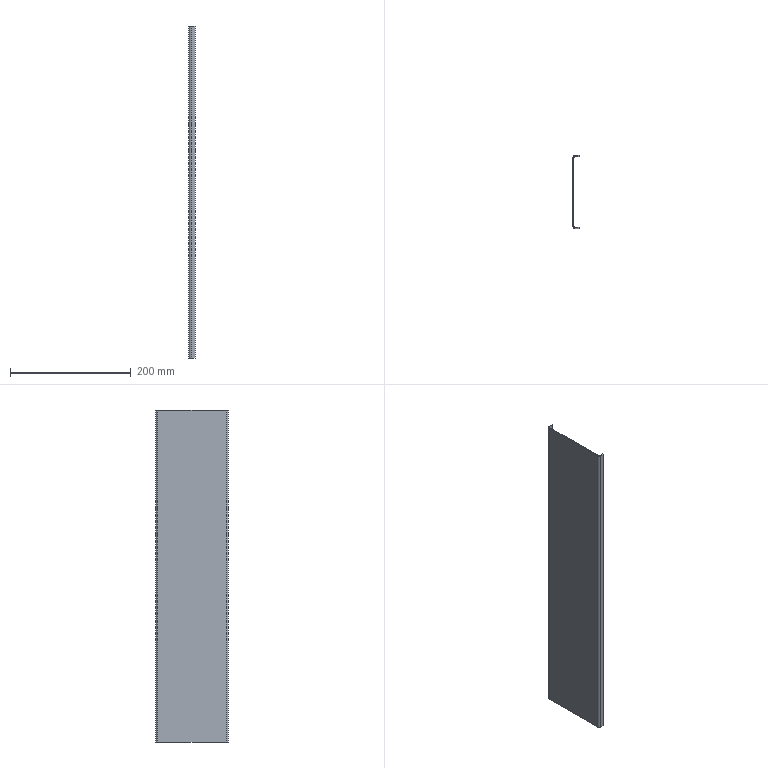Part | STEP file | SYL_0392D6J1SYL0380DJ100-324063 | 1 solid | 22 faces | box 10 x 120 x 550 mm | volume 111077 mm3 | plane 18 | cylinder 4 | commonest cylinder face diameters 4 x2 7 x2
STEP:
#1=CARTESIAN_POINT('',(5.,60.,-275.));
#2=VERTEX_POINT('',#1);
#3=CARTESIAN_POINT('',(5.,58.5,-275.));
#4=VERTEX_POINT('',#3);
#5=CARTESIAN_POINT('',(5.,58.5,-275.));
#6=DIRECTION('',(0.,-1.,0.));
#7=VECTOR('',#6,1000.);
#8=LINE('',#5,#7);
#9=EDGE_CURVE('',#2,#4,#8,.T.);
#10=ORIENTED_EDGE('',*,*,#9,.F.);
#11=CARTESIAN_POINT('',(5.,60.,275.));
#12=VERTEX_POINT('',#11);
#13=CARTESIAN_POINT('',(5.,60.,-275.));
#14=DIRECTION('',(0.,0.,-1.));
#15=VECTOR('',#14,1000.);
#16=LINE('',#13,#15);
#17=EDGE_CURVE('',#12,#2,#16,.T.);
#18=ORIENTED_EDGE('',*,*,#17,.F.);
#19=CARTESIAN_POINT('',(5.,58.5,275.));
#20=VERTEX_POINT('',#19);
#21=CARTESIAN_POINT('',(5.,58.5,275.));
#22=DIRECTION('',(0.,-1.,0.));
#23=VECTOR('',#22,1000.);
#24=LINE('',#21,#23);
#25=EDGE_CURVE('',#12,#20,#24,.T.);
#26=ORIENTED_EDGE('',*,*,#25,.T.);
#27=CARTESIAN_POINT('',(5.,58.5,275.));
#28=DIRECTION('',(0.,0.,-1.));
#29=VECTOR('',#28,1000.);
#30=LINE('',#27,#29);
#31=EDGE_CURVE('',#20,#4,#30,.T.);
#32=ORIENTED_EDGE('',*,*,#31,.T.);
#33=EDGE_LOOP('',(#10,#18,#26,#32));
#34=FACE_OUTER_BOUND('',#33,.T.);
#35=CARTESIAN_POINT('',(5.,58.5,275.));
#36=DIRECTION('',(1.,0.,0.));
#37=DIRECTION('',(0.,0.,-1.));
#38=AXIS2_PLACEMENT_3D('',#35,#36,#37);
#39=PLANE('',#38);
#40=ADVANCED_FACE('',(#34),#39,.T.);
#41=ORIENTED_EDGE('',*,*,#25,.F.);
#42=CARTESIAN_POINT('',(-1.5,60.,275.));
#43=VERTEX_POINT('',#42);
#44=CARTESIAN_POINT('',(5.,60.,275.));
#45=DIRECTION('',(1.,0.,0.));
#46=VECTOR('',#45,1000.);
#47=LINE('',#44,#46);
#48=EDGE_CURVE('',#43,#12,#47,.T.);
#49=ORIENTED_EDGE('',*,*,#48,.F.);
#50=CARTESIAN_POINT('',(-1.5,58.5,275.));
#51=VERTEX_POINT('',#50);
#52=CARTESIAN_POINT('',(-1.5,58.5,275.));
#53=DIRECTION('',(0.,-1.,0.));
#54=VECTOR('',#53,1000.);
#55=LINE('',#52,#54);
#56=EDGE_CURVE('',#43,#51,#55,.T.);
#57=ORIENTED_EDGE('',*,*,#56,.T.);
#58=CARTESIAN_POINT('',(-1.5,58.5,275.));
#59=DIRECTION('',(1.,0.,0.));
#60=VECTOR('',#59,1000.);
#61=LINE('',#58,#60);
#62=EDGE_CURVE('',#51,#20,#61,.T.);
#63=ORIENTED_EDGE('',*,*,#62,.T.);
#64=EDGE_LOOP('',(#41,#49,#57,#63));
#65=FACE_OUTER_BOUND('',#64,.T.);
#66=CARTESIAN_POINT('',(-1.5,58.5,275.));
#67=DIRECTION('',(0.,0.,1.));
#68=DIRECTION('',(1.,0.,0.));
#69=AXIS2_PLACEMENT_3D('',#66,#67,#68);
#70=PLANE('',#69);
#71=ADVANCED_FACE('',(#65),#70,.T.);
#72=ORIENTED_EDGE('',*,*,#56,.F.);
#73=CARTESIAN_POINT('',(-5.,56.5,275.));
#74=VERTEX_POINT('',#73);
#75=CARTESIAN_POINT('',(-1.5,56.5,275.));
#76=DIRECTION('',(0.,0.,-1.));
#77=DIRECTION('',(-1.,0.,0.));
#78=AXIS2_PLACEMENT_3D('',#75,#76,#77);
#79=CIRCLE('',#78,3.5);
#80=EDGE_CURVE('',#74,#43,#79,.T.);
#81=ORIENTED_EDGE('',*,*,#80,.F.);
#82=CARTESIAN_POINT('',(-3.5,56.5,275.));
#83=VERTEX_POINT('',#82);
#84=CARTESIAN_POINT('',(-3.5,56.5,275.));
#85=DIRECTION('',(1.,0.,0.));
#86=VECTOR('',#85,1000.);
#87=LINE('',#84,#86);
#88=EDGE_CURVE('',#74,#83,#87,.T.);
#89=ORIENTED_EDGE('',*,*,#88,.T.);
#90=CARTESIAN_POINT('',(-1.5,56.5,275.));
#91=DIRECTION('',(0.,0.,-1.));
#92=DIRECTION('',(-1.,0.,0.));
#93=AXIS2_PLACEMENT_3D('',#90,#91,#92);
#94=CIRCLE('',#93,2.);
#95=EDGE_CURVE('',#83,#51,#94,.T.);
#96=ORIENTED_EDGE('',*,*,#95,.T.);
#97=EDGE_LOOP('',(#72,#81,#89,#96));
#98=FACE_OUTER_BOUND('',#97,.T.);
#99=CARTESIAN_POINT('',(-1.5,56.5,275.));
#100=DIRECTION('',(0.,0.,1.));
#101=DIRECTION('',(1.,0.,0.));
#102=AXIS2_PLACEMENT_3D('',#99,#100,#101);
#103=PLANE('',#102);
#104=ADVANCED_FACE('',(#98),#103,.T.);
#105=ORIENTED_EDGE('',*,*,#88,.F.);
#106=CARTESIAN_POINT('',(-5.,-56.5,275.));
#107=VERTEX_POINT('',#106);
#108=CARTESIAN_POINT('',(-5.,60.,275.));
#109=DIRECTION('',(0.,1.,0.));
#110=VECTOR('',#109,1000.);
#111=LINE('',#108,#110);
#112=EDGE_CURVE('',#107,#74,#111,.T.);
#113=ORIENTED_EDGE('',*,*,#112,.F.);
#114=CARTESIAN_POINT('',(-3.5,-56.5,275.));
#115=VERTEX_POINT('',#114);
#116=CARTESIAN_POINT('',(-3.5,-56.5,275.));
#117=DIRECTION('',(1.,0.,0.));
#118=VECTOR('',#117,1000.);
#119=LINE('',#116,#118);
#120=EDGE_CURVE('',#107,#115,#119,.T.);
#121=ORIENTED_EDGE('',*,*,#120,.T.);
#122=CARTESIAN_POINT('',(-3.5,-56.5,275.));
#123=DIRECTION('',(0.,1.,0.));
#124=VECTOR('',#123,1000.);
#125=LINE('',#122,#124);
#126=EDGE_CURVE('',#115,#83,#125,.T.);
#127=ORIENTED_EDGE('',*,*,#126,.T.);
#128=EDGE_LOOP('',(#105,#113,#121,#127));
#129=FACE_OUTER_BOUND('',#128,.T.);
#130=CARTESIAN_POINT('',(-3.5,-56.5,275.));
#131=DIRECTION('',(0.,0.,1.));
#132=DIRECTION('',(0.,1.,0.));
#133=AXIS2_PLACEMENT_3D('',#130,#131,#132);
#134=PLANE('',#133);
#135=ADVANCED_FACE('',(#129),#134,.T.);
#136=ORIENTED_EDGE('',*,*,#120,.F.);
#137=CARTESIAN_POINT('',(-1.5,-60.,275.));
#138=VERTEX_POINT('',#137);
#139=CARTESIAN_POINT('',(-1.5,-56.5,275.));
#140=DIRECTION('',(0.,0.,-1.));
#141=DIRECTION('',(-1.,0.,0.));
#142=AXIS2_PLACEMENT_3D('',#139,#140,#141);
#143=CIRCLE('',#142,3.5);
#144=EDGE_CURVE('',#138,#107,#143,.T.);
#145=ORIENTED_EDGE('',*,*,#144,.F.);
#146=CARTESIAN_POINT('',(-1.5,-58.5,275.));
#147=VERTEX_POINT('',#146);
#148=CARTESIAN_POINT('',(-1.5,-58.5,275.));
#149=DIRECTION('',(0.,1.,0.));
#150=VECTOR('',#149,1000.);
#151=LINE('',#148,#150);
#152=EDGE_CURVE('',#138,#147,#151,.T.);
#153=ORIENTED_EDGE('',*,*,#152,.T.);
#154=CARTESIAN_POINT('',(-1.5,-56.5,275.));
#155=DIRECTION('',(0.,0.,-1.));
#156=DIRECTION('',(0.,-1.,0.));
#157=AXIS2_PLACEMENT_3D('',#154,#155,#156);
#158=CIRCLE('',#157,2.);
#159=EDGE_CURVE('',#147,#115,#158,.T.);
#160=ORIENTED_EDGE('',*,*,#159,.T.);
#161=EDGE_LOOP('',(#136,#145,#153,#160));
#162=FACE_OUTER_BOUND('',#161,.T.);
#163=CARTESIAN_POINT('',(-1.5,-56.5,275.));
#164=DIRECTION('',(0.,0.,1.));
#165=DIRECTION('',(1.,0.,0.));
#166=AXIS2_PLACEMENT_3D('',#163,#164,#165);
#167=PLANE('',#166);
#168=ADVANCED_FACE('',(#162),#167,.T.);
#169=ORIENTED_EDGE('',*,*,#152,.F.);
#170=CARTESIAN_POINT('',(5.,-60.,275.));
#171=VERTEX_POINT('',#170);
#172=CARTESIAN_POINT('',(-5.,-60.,275.));
#173=DIRECTION('',(-1.,0.,0.));
#174=VECTOR('',#173,1000.);
#175=LINE('',#172,#174);
#176=EDGE_CURVE('',#171,#138,#175,.T.);
#177=ORIENTED_EDGE('',*,*,#176,.F.);
#178=CARTESIAN_POINT('',(5.,-58.5,275.));
#179=VERTEX_POINT('',#178);
#180=CARTESIAN_POINT('',(5.,-58.5,275.));
#181=DIRECTION('',(0.,1.,0.));
#182=VECTOR('',#181,1000.);
#183=LINE('',#180,#182);
#184=EDGE_CURVE('',#171,#179,#183,.T.);
#185=ORIENTED_EDGE('',*,*,#184,.T.);
#186=CARTESIAN_POINT('',(5.,-58.5,275.));
#187=DIRECTION('',(-1.,0.,0.));
#188=VECTOR('',#187,1000.);
#189=LINE('',#186,#188);
#190=EDGE_CURVE('',#179,#147,#189,.T.);
#191=ORIENTED_EDGE('',*,*,#190,.T.);
#192=EDGE_LOOP('',(#169,#177,#185,#191));
#193=FACE_OUTER_BOUND('',#192,.T.);
#194=CARTESIAN_POINT('',(5.,-58.5,275.));
#195=DIRECTION('',(0.,0.,1.));
#196=DIRECTION('',(-1.,0.,0.));
#197=AXIS2_PLACEMENT_3D('',#194,#195,#196);
#198=PLANE('',#197);
#199=ADVANCED_FACE('',(#193),#198,.T.);
#200=ORIENTED_EDGE('',*,*,#184,.F.);
#201=CARTESIAN_POINT('',(5.,-60.,-275.));
#202=VERTEX_POINT('',#201);
#203=CARTESIAN_POINT('',(5.,-60.,-275.));
#204=DIRECTION('',(0.,0.,-1.));
#205=VECTOR('',#204,1000.);
#206=LINE('',#203,#205);
#207=EDGE_CURVE('',#171,#202,#206,.T.);
#208=ORIENTED_EDGE('',*,*,#207,.T.);
#209=CARTESIAN_POINT('',(5.,-58.5,-275.));
#210=VERTEX_POINT('',#209);
#211=CARTESIAN_POINT('',(5.,-58.5,-275.));
#212=DIRECTION('',(0.,1.,0.));
#213=VECTOR('',#212,1000.);
#214=LINE('',#211,#213);
#215=EDGE_CURVE('',#202,#210,#214,.T.);
#216=ORIENTED_EDGE('',*,*,#215,.T.);
#217=CARTESIAN_POINT('',(5.,-58.5,275.));
#218=DIRECTION('',(0.,0.,-1.));
#219=VECTOR('',#218,1000.);
#220=LINE('',#217,#219);
#221=EDGE_CURVE('',#179,#210,#220,.T.);
#222=ORIENTED_EDGE('',*,*,#221,.F.);
#223=EDGE_LOOP('',(#200,#208,#216,#222));
#224=FACE_OUTER_BOUND('',#223,.T.);
#225=CARTESIAN_POINT('',(5.,-58.5,275.));
#226=DIRECTION('',(-1.,0.,0.));
#227=DIRECTION('',(0.,0.,-1.));
#228=AXIS2_PLACEMENT_3D('',#225,#226,#227);
#229=PLANE('',#228);
#230=ADVANCED_FACE('',(#224),#229,.F.);
#231=ORIENTED_EDGE('',*,*,#215,.F.);
#232=CARTESIAN_POINT('',(-1.5,-60.,-275.));
#233=VERTEX_POINT('',#232);
#234=CARTESIAN_POINT('',(-5.,-60.,-275.));
#235=DIRECTION('',(-1.,0.,0.));
#236=VECTOR('',#235,1000.);
#237=LINE('',#234,#236);
#238=EDGE_CURVE('',#202,#233,#237,.T.);
#239=ORIENTED_EDGE('',*,*,#238,.T.);
#240=CARTESIAN_POINT('',(-1.5,-58.5,-275.));
#241=VERTEX_POINT('',#240);
#242=CARTESIAN_POINT('',(-1.5,-58.5,-275.));
#243=DIRECTION('',(0.,1.,0.));
#244=VECTOR('',#243,1000.);
#245=LINE('',#242,#244);
#246=EDGE_CURVE('',#233,#241,#245,.T.);
#247=ORIENTED_EDGE('',*,*,#246,.T.);
#248=CARTESIAN_POINT('',(5.,-58.5,-275.));
#249=DIRECTION('',(-1.,0.,0.));
#250=VECTOR('',#249,1000.);
#251=LINE('',#248,#250);
#252=EDGE_CURVE('',#210,#241,#251,.T.);
#253=ORIENTED_EDGE('',*,*,#252,.F.);
#254=EDGE_LOOP('',(#231,#239,#247,#253));
#255=FACE_OUTER_BOUND('',#254,.T.);
#256=CARTESIAN_POINT('',(5.,-58.5,-275.));
#257=DIRECTION('',(0.,0.,1.));
#258=DIRECTION('',(-1.,0.,0.));
#259=AXIS2_PLACEMENT_3D('',#256,#257,#258);
#260=PLANE('',#259);
#261=ADVANCED_FACE('',(#255),#260,.F.);
#262=ORIENTED_EDGE('',*,*,#246,.F.);
#263=CARTESIAN_POINT('',(-5.,-56.5,-275.));
#264=VERTEX_POINT('',#263);
#265=CARTESIAN_POINT('',(-1.5,-56.5,-275.));
#266=DIRECTION('',(0.,0.,1.));
#267=DIRECTION('',(-1.,0.,0.));
#268=AXIS2_PLACEMENT_3D('',#265,#266,#267);
#269=CIRCLE('',#268,3.5);
#270=EDGE_CURVE('',#264,#233,#269,.T.);
#271=ORIENTED_EDGE('',*,*,#270,.F.);
#272=CARTESIAN_POINT('',(-3.5,-56.5,-275.));
#273=VERTEX_POINT('',#272);
#274=CARTESIAN_POINT('',(-3.5,-56.5,-275.));
#275=DIRECTION('',(1.,0.,0.));
#276=VECTOR('',#275,1000.);
#277=LINE('',#274,#276);
#278=EDGE_CURVE('',#264,#273,#277,.T.);
#279=ORIENTED_EDGE('',*,*,#278,.T.);
#280=CARTESIAN_POINT('',(-1.5,-56.5,-275.));
#281=DIRECTION('',(0.,0.,1.));
#282=DIRECTION('',(-1.,0.,0.));
#283=AXIS2_PLACEMENT_3D('',#280,#281,#282);
#284=CIRCLE('',#283,2.);
#285=EDGE_CURVE('',#273,#241,#284,.T.);
#286=ORIENTED_EDGE('',*,*,#285,.T.);
#287=EDGE_LOOP('',(#262,#271,#279,#286));
#288=FACE_OUTER_BOUND('',#287,.T.);
#289=CARTESIAN_POINT('',(-1.5,-56.5,-275.));
#290=DIRECTION('',(0.,0.,-1.));
#291=DIRECTION('',(-1.,0.,0.));
#292=AXIS2_PLACEMENT_3D('',#289,#290,#291);
#293=PLANE('',#292);
#294=ADVANCED_FACE('',(#288),#293,.T.);
#295=ORIENTED_EDGE('',*,*,#278,.F.);
#296=CARTESIAN_POINT('',(-5.,56.5,-275.));
#297=VERTEX_POINT('',#296);
#298=CARTESIAN_POINT('',(-5.,60.,-275.));
#299=DIRECTION('',(0.,1.,0.));
#300=VECTOR('',#299,1000.);
#301=LINE('',#298,#300);
#302=EDGE_CURVE('',#264,#297,#301,.T.);
#303=ORIENTED_EDGE('',*,*,#302,.T.);
#304=CARTESIAN_POINT('',(-3.5,56.5,-275.));
#305=VERTEX_POINT('',#304);
#306=CARTESIAN_POINT('',(-3.5,56.5,-275.));
#307=DIRECTION('',(1.,0.,0.));
#308=VECTOR('',#307,1000.);
#309=LINE('',#306,#308);
#310=EDGE_CURVE('',#297,#305,#309,.T.);
#311=ORIENTED_EDGE('',*,*,#310,.T.);
#312=CARTESIAN_POINT('',(-3.5,-56.5,-275.));
#313=DIRECTION('',(0.,1.,0.));
#314=VECTOR('',#313,1000.);
#315=LINE('',#312,#314);
#316=EDGE_CURVE('',#273,#305,#315,.T.);
#317=ORIENTED_EDGE('',*,*,#316,.F.);
#318=EDGE_LOOP('',(#295,#303,#311,#317));
#319=FACE_OUTER_BOUND('',#318,.T.);
#320=CARTESIAN_POINT('',(-3.5,-56.5,-275.));
#321=DIRECTION('',(0.,0.,1.));
#322=DIRECTION('',(0.,1.,0.));
#323=AXIS2_PLACEMENT_3D('',#320,#321,#322);
#324=PLANE('',#323);
#325=ADVANCED_FACE('',(#319),#324,.F.);
#326=ORIENTED_EDGE('',*,*,#310,.F.);
#327=CARTESIAN_POINT('',(-1.5,60.,-275.));
#328=VERTEX_POINT('',#327);
#329=CARTESIAN_POINT('',(-1.5,56.5,-275.));
#330=DIRECTION('',(0.,0.,1.));
#331=DIRECTION('',(-1.,0.,0.));
#332=AXIS2_PLACEMENT_3D('',#329,#330,#331);
#333=CIRCLE('',#332,3.5);
#334=EDGE_CURVE('',#328,#297,#333,.T.);
#335=ORIENTED_EDGE('',*,*,#334,.F.);
#336=CARTESIAN_POINT('',(-1.5,58.5,-275.));
#337=VERTEX_POINT('',#336);
#338=CARTESIAN_POINT('',(-1.5,58.5,-275.));
#339=DIRECTION('',(0.,-1.,0.));
#340=VECTOR('',#339,1000.);
#341=LINE('',#338,#340);
#342=EDGE_CURVE('',#328,#337,#341,.T.);
#343=ORIENTED_EDGE('',*,*,#342,.T.);
#344=CARTESIAN_POINT('',(-1.5,56.5,-275.));
#345=DIRECTION('',(0.,0.,1.));
#346=DIRECTION('',(0.,1.,0.));
#347=AXIS2_PLACEMENT_3D('',#344,#345,#346);
#348=CIRCLE('',#347,2.);
#349=EDGE_CURVE('',#337,#305,#348,.T.);
#350=ORIENTED_EDGE('',*,*,#349,.T.);
#351=EDGE_LOOP('',(#326,#335,#343,#350));
#352=FACE_OUTER_BOUND('',#351,.T.);
#353=CARTESIAN_POINT('',(-1.5,56.5,-275.));
#354=DIRECTION('',(0.,0.,-1.));
#355=DIRECTION('',(-1.,0.,0.));
#356=AXIS2_PLACEMENT_3D('',#353,#354,#355);
#357=PLANE('',#356);
#358=ADVANCED_FACE('',(#352),#357,.T.);
#359=CARTESIAN_POINT('',(5.,60.,-275.));
#360=DIRECTION('',(1.,0.,0.));
#361=VECTOR('',#360,1000.);
#362=LINE('',#359,#361);
#363=EDGE_CURVE('',#328,#2,#362,.T.);
#364=ORIENTED_EDGE('',*,*,#363,.T.);
#365=ORIENTED_EDGE('',*,*,#9,.T.);
#366=CARTESIAN_POINT('',(-1.5,58.5,-275.));
#367=DIRECTION('',(1.,0.,0.));
#368=VECTOR('',#367,1000.);
#369=LINE('',#366,#368);
#370=EDGE_CURVE('',#337,#4,#369,.T.);
#371=ORIENTED_EDGE('',*,*,#370,.F.);
#372=ORIENTED_EDGE('',*,*,#342,.F.);
#373=EDGE_LOOP('',(#364,#365,#371,#372));
#374=FACE_OUTER_BOUND('',#373,.T.);
#375=CARTESIAN_POINT('',(-1.5,58.5,-275.));
#376=DIRECTION('',(0.,0.,1.));
#377=DIRECTION('',(1.,0.,0.));
#378=AXIS2_PLACEMENT_3D('',#375,#376,#377);
#379=PLANE('',#378);
#380=ADVANCED_FACE('',(#374),#379,.F.);
#381=ORIENTED_EDGE('',*,*,#349,.F.);
#382=CARTESIAN_POINT('',(-1.5,58.5,-275.));
#383=DIRECTION('',(0.,0.,1.));
#384=VECTOR('',#383,1000.);
#385=LINE('',#382,#384);
#386=EDGE_CURVE('',#337,#51,#385,.T.);
#387=ORIENTED_EDGE('',*,*,#386,.T.);
#388=ORIENTED_EDGE('',*,*,#95,.F.);
#389=CARTESIAN_POINT('',(-3.5,56.5,275.));
#390=DIRECTION('',(0.,0.,-1.));
#391=VECTOR('',#390,1000.);
#392=LINE('',#389,#391);
#393=EDGE_CURVE('',#83,#305,#392,.T.);
#394=ORIENTED_EDGE('',*,*,#393,.T.);
#395=EDGE_LOOP('',(#381,#387,#388,#394));
#396=FACE_OUTER_BOUND('',#395,.T.);
#397=CARTESIAN_POINT('',(-1.5,56.5,991.98));
#398=DIRECTION('',(0.,0.,-1.));
#399=DIRECTION('',(-1.,0.,0.));
#400=AXIS2_PLACEMENT_3D('',#397,#398,#399);
#401=CYLINDRICAL_SURFACE('',#400,2.);
#402=ADVANCED_FACE('',(#396),#401,.F.);
#403=ORIENTED_EDGE('',*,*,#62,.F.);
#404=ORIENTED_EDGE('',*,*,#386,.F.);
#405=ORIENTED_EDGE('',*,*,#370,.T.);
#406=ORIENTED_EDGE('',*,*,#31,.F.);
#407=EDGE_LOOP('',(#403,#404,#405,#406));
#408=FACE_OUTER_BOUND('',#407,.T.);
#409=CARTESIAN_POINT('',(5.,58.5,-275.));
#410=DIRECTION('',(0.,1.,0.));
#411=DIRECTION('',(1.,0.,0.));
#412=AXIS2_PLACEMENT_3D('',#409,#410,#411);
#413=PLANE('',#412);
#414=ADVANCED_FACE('',(#408),#413,.F.);
#415=ORIENTED_EDGE('',*,*,#285,.F.);
#416=CARTESIAN_POINT('',(-3.5,-56.5,-275.));
#417=DIRECTION('',(0.,0.,1.));
#418=VECTOR('',#417,1000.);
#419=LINE('',#416,#418);
#420=EDGE_CURVE('',#273,#115,#419,.T.);
#421=ORIENTED_EDGE('',*,*,#420,.T.);
#422=ORIENTED_EDGE('',*,*,#159,.F.);
#423=CARTESIAN_POINT('',(-1.5,-58.5,275.));
#424=DIRECTION('',(0.,0.,-1.));
#425=VECTOR('',#424,1000.);
#426=LINE('',#423,#425);
#427=EDGE_CURVE('',#147,#241,#426,.T.);
#428=ORIENTED_EDGE('',*,*,#427,.T.);
#429=EDGE_LOOP('',(#415,#421,#422,#428));
#430=FACE_OUTER_BOUND('',#429,.T.);
#431=CARTESIAN_POINT('',(-1.5,-56.5,991.98));
#432=DIRECTION('',(0.,0.,-1.));
#433=DIRECTION('',(-1.,0.,0.));
#434=AXIS2_PLACEMENT_3D('',#431,#432,#433);
#435=CYLINDRICAL_SURFACE('',#434,2.);
#436=ADVANCED_FACE('',(#430),#435,.F.);
#437=ORIENTED_EDGE('',*,*,#252,.T.);
#438=ORIENTED_EDGE('',*,*,#427,.F.);
#439=ORIENTED_EDGE('',*,*,#190,.F.);
#440=ORIENTED_EDGE('',*,*,#221,.T.);
#441=EDGE_LOOP('',(#437,#438,#439,#440));
#442=FACE_OUTER_BOUND('',#441,.T.);
#443=CARTESIAN_POINT('',(-5.,-58.5,-275.));
#444=DIRECTION('',(0.,-1.,0.));
#445=DIRECTION('',(0.,0.,-1.));
#446=AXIS2_PLACEMENT_3D('',#443,#444,#445);
#447=PLANE('',#446);
#448=ADVANCED_FACE('',(#442),#447,.F.);
#449=ORIENTED_EDGE('',*,*,#126,.F.);
#450=ORIENTED_EDGE('',*,*,#420,.F.);
#451=ORIENTED_EDGE('',*,*,#316,.T.);
#452=ORIENTED_EDGE('',*,*,#393,.F.);
#453=EDGE_LOOP('',(#449,#450,#451,#452));
#454=FACE_OUTER_BOUND('',#453,.T.);
#455=CARTESIAN_POINT('',(-3.5,60.,-275.));
#456=DIRECTION('',(-1.,0.,0.));
#457=DIRECTION('',(0.,0.,1.));
#458=AXIS2_PLACEMENT_3D('',#455,#456,#457);
#459=PLANE('',#458);
#460=ADVANCED_FACE('',(#454),#459,.F.);
#461=ORIENTED_EDGE('',*,*,#334,.T.);
#462=CARTESIAN_POINT('',(-5.,56.5,991.98));
#463=DIRECTION('',(0.,0.,-1.));
#464=VECTOR('',#463,1000.);
#465=LINE('',#462,#464);
#466=EDGE_CURVE('',#74,#297,#465,.T.);
#467=ORIENTED_EDGE('',*,*,#466,.F.);
#468=ORIENTED_EDGE('',*,*,#80,.T.);
#469=CARTESIAN_POINT('',(-1.5,60.,991.98));
#470=DIRECTION('',(0.,0.,1.));
#471=VECTOR('',#470,1000.);
#472=LINE('',#469,#471);
#473=EDGE_CURVE('',#328,#43,#472,.T.);
#474=ORIENTED_EDGE('',*,*,#473,.F.);
#475=EDGE_LOOP('',(#461,#467,#468,#474));
#476=FACE_OUTER_BOUND('',#475,.T.);
#477=CARTESIAN_POINT('',(-1.5,56.5,991.98));
#478=DIRECTION('',(0.,0.,-1.));
#479=DIRECTION('',(-1.,0.,0.));
#480=AXIS2_PLACEMENT_3D('',#477,#478,#479);
#481=CYLINDRICAL_SURFACE('',#480,3.5);
#482=ADVANCED_FACE('',(#476),#481,.T.);
#483=ORIENTED_EDGE('',*,*,#48,.T.);
#484=ORIENTED_EDGE('',*,*,#17,.T.);
#485=ORIENTED_EDGE('',*,*,#363,.F.);
#486=ORIENTED_EDGE('',*,*,#473,.T.);
#487=EDGE_LOOP('',(#483,#484,#485,#486));
#488=FACE_OUTER_BOUND('',#487,.T.);
#489=CARTESIAN_POINT('',(5.,60.,-275.));
#490=DIRECTION('',(0.,1.,0.));
#491=DIRECTION('',(1.,0.,0.));
#492=AXIS2_PLACEMENT_3D('',#489,#490,#491);
#493=PLANE('',#492);
#494=ADVANCED_FACE('',(#488),#493,.T.);
#495=ORIENTED_EDGE('',*,*,#270,.T.);
#496=CARTESIAN_POINT('',(-1.5,-60.,991.98));
#497=DIRECTION('',(0.,0.,-1.));
#498=VECTOR('',#497,1000.);
#499=LINE('',#496,#498);
#500=EDGE_CURVE('',#138,#233,#499,.T.);
#501=ORIENTED_EDGE('',*,*,#500,.F.);
#502=ORIENTED_EDGE('',*,*,#144,.T.);
#503=CARTESIAN_POINT('',(-5.,-56.5,991.98));
#504=DIRECTION('',(0.,0.,1.));
#505=VECTOR('',#504,1000.);
#506=LINE('',#503,#505);
#507=EDGE_CURVE('',#264,#107,#506,.T.);
#508=ORIENTED_EDGE('',*,*,#507,.F.);
#509=EDGE_LOOP('',(#495,#501,#502,#508));
#510=FACE_OUTER_BOUND('',#509,.T.);
#511=CARTESIAN_POINT('',(-1.5,-56.5,991.98));
#512=DIRECTION('',(0.,0.,-1.));
#513=DIRECTION('',(-1.,0.,0.));
#514=AXIS2_PLACEMENT_3D('',#511,#512,#513);
#515=CYLINDRICAL_SURFACE('',#514,3.5);
#516=ADVANCED_FACE('',(#510),#515,.T.);
#517=ORIENTED_EDGE('',*,*,#238,.F.);
#518=ORIENTED_EDGE('',*,*,#207,.F.);
#519=ORIENTED_EDGE('',*,*,#176,.T.);
#520=ORIENTED_EDGE('',*,*,#500,.T.);
#521=EDGE_LOOP('',(#517,#518,#519,#520));
#522=FACE_OUTER_BOUND('',#521,.T.);
#523=CARTESIAN_POINT('',(-5.,-60.,-275.));
#524=DIRECTION('',(0.,-1.,0.));
#525=DIRECTION('',(0.,0.,-1.));
#526=AXIS2_PLACEMENT_3D('',#523,#524,#525);
#527=PLANE('',#526);
#528=ADVANCED_FACE('',(#522),#527,.T.);
#529=ORIENTED_EDGE('',*,*,#112,.T.);
#530=ORIENTED_EDGE('',*,*,#466,.T.);
#531=ORIENTED_EDGE('',*,*,#302,.F.);
#532=ORIENTED_EDGE('',*,*,#507,.T.);
#533=EDGE_LOOP('',(#529,#530,#531,#532));
#534=FACE_OUTER_BOUND('',#533,.T.);
#535=CARTESIAN_POINT('',(-5.,60.,-275.));
#536=DIRECTION('',(-1.,0.,0.));
#537=DIRECTION('',(0.,0.,1.));
#538=AXIS2_PLACEMENT_3D('',#535,#536,#537);
#539=PLANE('',#538);
#540=ADVANCED_FACE('',(#534),#539,.T.);
#541=CLOSED_SHELL('',(#40,#71,#104,#135,#168,#199,#230,#261,#294,#325,#358,#380,#402,#414,#436,#448,#460,#482,#494,#516,#528,#540));
#542=MANIFOLD_SOLID_BREP('',#541);
#543=CARTESIAN_POINT('',(0.,0.,0.));
#544=DIRECTION('',(0.,0.,1.));
#545=DIRECTION('',(1.,0.,0.));
#546=AXIS2_PLACEMENT_3D('',#543,#544,#545);
#547=(LENGTH_UNIT()NAMED_UNIT(*)SI_UNIT(.MILLI.,.METRE.));
#548=UNCERTAINTY_MEASURE_WITH_UNIT(LENGTH_MEASURE(0.00001),#547,'','');
#549=(NAMED_UNIT(*)PLANE_ANGLE_UNIT()SI_UNIT($,.RADIAN.));
#550=(NAMED_UNIT(*)SI_UNIT($,.STERADIAN.)SOLID_ANGLE_UNIT());
#551=(GEOMETRIC_REPRESENTATION_CONTEXT(3)GLOBAL_UNCERTAINTY_ASSIGNED_CONTEXT((#548))GLOBAL_UNIT_ASSIGNED_CONTEXT((#547,#549,#550))REPRESENTATION_CONTEXT('',''));
#552=ADVANCED_BREP_SHAPE_REPRESENTATION('',(#542,#546),#551);